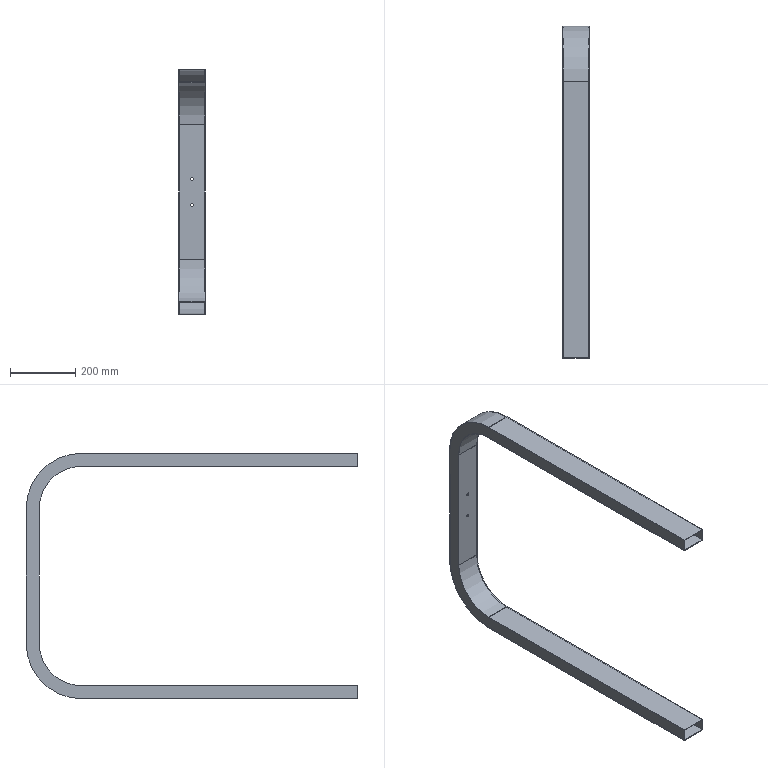Part | STEP file | 6100201R | 1 solid | 31 faces | box 80 x 1020 x 755 mm | volume 1103888 mm3 | plane 18 | cylinder 13 | commonest cylinder face diameters 9 x4 260 x2 264 x2 336 x2 340 x2 40 x1